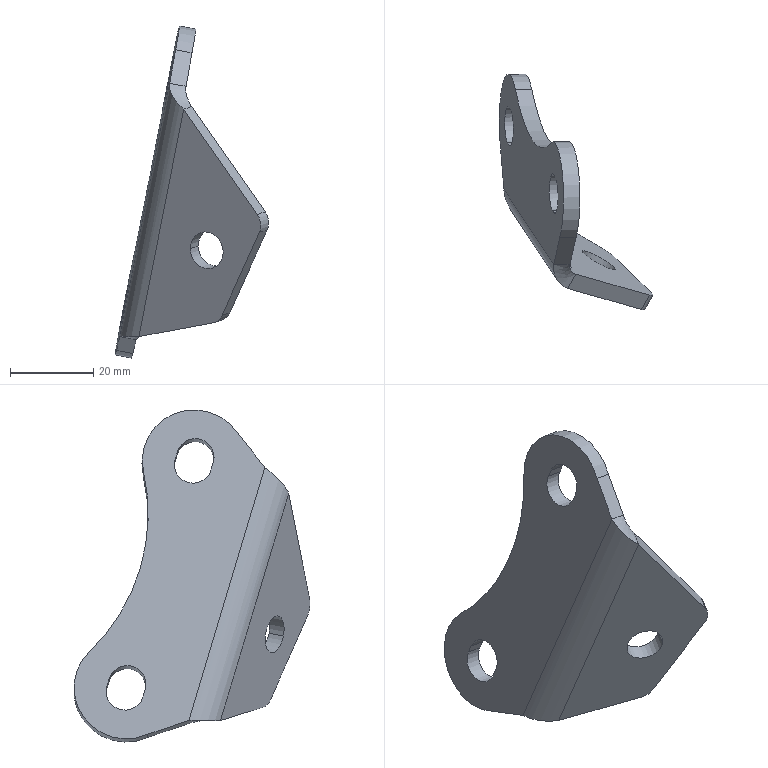Part | SolidWorks | features BaseBody 1 | 1 solid | 28 faces | box 36.914 x 56.808 x 79.896 mm | volume 12706 mm3 | plane 13 | cylinder 13 | spline 2 | commonest cylinder face diameters 9 x6 8 x3 25 x2 16 x1 94.633 x1
STEP:
#1=CARTESIAN_POINT('',(96.44,489.599,-664.758));
#2=VERTEX_POINT('',#1);
#3=CARTESIAN_POINT('',(96.779,498.232,-662.234));
#4=VERTEX_POINT('',#3);
#5=CARTESIAN_POINT('',(96.61,493.916,-663.496));
#6=DIRECTION('',(0.982,0.01648,-0.1883));
#7=DIRECTION('',(-0.03769,-0.9591,-0.2804));
#8=AXIS2_PLACEMENT_3D('',#5,#6,#7);
#9=CIRCLE('',#8,4.5);
#10=EDGE_CURVE('',#2,#4,#9,.T.);
#11=ORIENTED_EDGE('',*,*,#10,.F.);
#12=CARTESIAN_POINT('',(96.811,489.035,-662.876));
#13=VERTEX_POINT('',#12);
#14=CARTESIAN_POINT('',(96.811,489.035,-662.876));
#15=DIRECTION('',(-0.1852,0.2825,-0.9412));
#16=VECTOR('',#15,1000.);
#17=LINE('',#14,#16);
#18=EDGE_CURVE('',#13,#2,#17,.T.);
#19=ORIENTED_EDGE('',*,*,#18,.F.);
#20=CARTESIAN_POINT('',(97.15,497.667,-660.352));
#21=VERTEX_POINT('',#20);
#22=CARTESIAN_POINT('',(96.98,493.351,-661.614));
#23=DIRECTION('',(0.982,0.01648,-0.1883));
#24=DIRECTION('',(0.03769,0.9591,0.2804));
#25=AXIS2_PLACEMENT_3D('',#22,#23,#24);
#26=CIRCLE('',#25,4.5);
#27=EDGE_CURVE('',#21,#13,#26,.T.);
#28=ORIENTED_EDGE('',*,*,#27,.F.);
#29=CARTESIAN_POINT('',(96.779,498.232,-662.234));
#30=DIRECTION('',(0.1852,-0.2825,0.9412));
#31=VECTOR('',#30,1000.);
#32=LINE('',#29,#31);
#33=EDGE_CURVE('',#4,#21,#32,.T.);
#34=ORIENTED_EDGE('',*,*,#33,.F.);
#35=EDGE_LOOP('',(#11,#19,#28,#34));
#36=FACE_BOUND('',#35,.T.);
#37=CARTESIAN_POINT('',(85.696,505.984,-719.349));
#38=VERTEX_POINT('',#37);
#39=CARTESIAN_POINT('',(86.035,514.616,-716.825));
#40=VERTEX_POINT('',#39);
#41=CARTESIAN_POINT('',(85.866,510.3,-718.087));
#42=DIRECTION('',(0.982,0.01648,-0.1883));
#43=DIRECTION('',(-0.03769,-0.9591,-0.2804));
#44=AXIS2_PLACEMENT_3D('',#41,#42,#43);
#45=CIRCLE('',#44,4.5);
#46=EDGE_CURVE('',#38,#40,#45,.T.);
#47=ORIENTED_EDGE('',*,*,#46,.F.);
#48=CARTESIAN_POINT('',(86.067,505.419,-717.466));
#49=VERTEX_POINT('',#48);
#50=CARTESIAN_POINT('',(86.067,505.419,-717.466));
#51=DIRECTION('',(-0.1852,0.2825,-0.9412));
#52=VECTOR('',#51,1000.);
#53=LINE('',#50,#52);
#54=EDGE_CURVE('',#49,#38,#53,.T.);
#55=ORIENTED_EDGE('',*,*,#54,.F.);
#56=CARTESIAN_POINT('',(86.406,514.051,-714.942));
#57=VERTEX_POINT('',#56);
#58=CARTESIAN_POINT('',(86.236,509.735,-716.204));
#59=DIRECTION('',(0.982,0.01648,-0.1883));
#60=DIRECTION('',(0.03769,0.9591,0.2804));
#61=AXIS2_PLACEMENT_3D('',#58,#59,#60);
#62=CIRCLE('',#61,4.5);
#63=EDGE_CURVE('',#57,#49,#62,.T.);
#64=ORIENTED_EDGE('',*,*,#63,.F.);
#65=CARTESIAN_POINT('',(86.035,514.616,-716.825));
#66=DIRECTION('',(0.1852,-0.2825,0.9412));
#67=VECTOR('',#66,1000.);
#68=LINE('',#65,#67);
#69=EDGE_CURVE('',#40,#57,#68,.T.);
#70=ORIENTED_EDGE('',*,*,#69,.F.);
#71=EDGE_LOOP('',(#47,#55,#64,#70));
#72=FACE_BOUND('',#71,.T.);
#73=CARTESIAN_POINT('',(83.998,504.784,-728.31));
#74=VERTEX_POINT('',#73);
#75=CARTESIAN_POINT('',(84.798,494.924,-725.));
#76=VERTEX_POINT('',#75);
#77=CARTESIAN_POINT('',(83.998,504.784,-728.31));
#78=DIRECTION('',(0.0767,-0.9452,0.3173));
#79=VECTOR('',#78,1000.);
#80=LINE('',#77,#79);
#81=EDGE_CURVE('',#74,#76,#80,.T.);
#82=ORIENTED_EDGE('',*,*,#81,.F.);
#83=CARTESIAN_POINT('',(87.586,518.791,-708.376));
#84=VERTEX_POINT('',#83);
#85=CARTESIAN_POINT('',(86.051,510.017,-717.145));
#86=DIRECTION('',(-0.982,-0.01648,0.1883));
#87=DIRECTION('',(0.1228,0.7019,0.7016));
#88=AXIS2_PLACEMENT_3D('',#85,#86,#87);
#89=CIRCLE('',#88,12.5);
#90=EDGE_CURVE('',#84,#74,#89,.T.);
#91=ORIENTED_EDGE('',*,*,#90,.F.);
#92=CARTESIAN_POINT('',(96.084,505.831,-665.193));
#93=VERTEX_POINT('',#92);
#94=CARTESIAN_POINT('',(93.395,552.004,-675.178));
#95=DIRECTION('',(0.982,0.01648,-0.1883));
#96=DIRECTION('',(0.05684,-0.9758,0.211));
#97=AXIS2_PLACEMENT_3D('',#94,#95,#96);
#98=CIRCLE('',#97,47.317);
#99=EDGE_CURVE('',#93,#84,#98,.T.);
#100=ORIENTED_EDGE('',*,*,#99,.F.);
#101=CARTESIAN_POINT('',(98.228,483.083,-656.006));
#102=VERTEX_POINT('',#101);
#103=CARTESIAN_POINT('',(96.795,493.633,-662.555));
#104=DIRECTION('',(-0.982,-0.01648,0.1883));
#105=DIRECTION('',(0.1146,-0.844,0.5239));
#106=AXIS2_PLACEMENT_3D('',#103,#104,#105);
#107=CIRCLE('',#106,12.5);
#108=EDGE_CURVE('',#102,#93,#107,.T.);
#109=ORIENTED_EDGE('',*,*,#108,.F.);
#110=CARTESIAN_POINT('',(96.787,476.64,-664.082));
#111=VERTEX_POINT('',#110);
#112=CARTESIAN_POINT('',(96.787,476.64,-664.082));
#113=DIRECTION('',(0.1381,0.6176,0.7742));
#114=VECTOR('',#113,1000.);
#115=LINE('',#112,#114);
#116=EDGE_CURVE('',#111,#102,#115,.T.);
#117=ORIENTED_EDGE('',*,*,#116,.F.);
#118=CARTESIAN_POINT('',(96.787,476.64,-664.082));
#119=DIRECTION('',(-0.1852,0.2825,-0.9412));
#120=VECTOR('',#119,1000.);
#121=LINE('',#118,#120);
#122=EDGE_CURVE('',#111,#76,#121,.T.);
#123=ORIENTED_EDGE('',*,*,#122,.T.);
#124=EDGE_LOOP('',(#82,#91,#100,#109,#117,#123));
#125=FACE_OUTER_BOUND('',#124,.T.);
#126=CARTESIAN_POINT('',(80.679,518.209,-744.441));
#127=DIRECTION('',(0.982,0.01648,-0.1883));
#128=DIRECTION('',(0.,-0.9962,-0.08716));
#129=AXIS2_PLACEMENT_3D('',#126,#127,#128);
#130=PLANE('',#129);
#131=ADVANCED_FACE('',(#36,#72,#125),#130,.T.);
#132=CARTESIAN_POINT('',(98.124,474.285,-668.916));
#133=VERTEX_POINT('',#132);
#134=CARTESIAN_POINT('',(98.124,474.285,-668.916));
#135=CARTESIAN_POINT('',(97.917,474.34,-668.601));
#136=CARTESIAN_POINT('',(97.535,474.506,-667.961));
#137=CARTESIAN_POINT('',(97.089,474.899,-666.982));
#138=CARTESIAN_POINT('',(96.798,475.41,-665.999));
#139=CARTESIAN_POINT('',(96.683,476.003,-665.026));
#140=CARTESIAN_POINT('',(96.731,476.427,-664.393));
#141=CARTESIAN_POINT('',(96.787,476.64,-664.082));
#142=B_SPLINE_CURVE_WITH_KNOTS('',3,(#134,#135,#136,#137,#138,#139,#140,#141),.UNSPECIFIED.,.F.,.F.,(4,1,1,1,1,4),(0.,0.2,0.4,0.6,0.8,1.),.UNSPECIFIED.);
#143=EDGE_CURVE('',#133,#111,#142,.T.);
#144=ORIENTED_EDGE('',*,*,#143,.F.);
#145=CARTESIAN_POINT('',(87.359,490.701,-723.614));
#146=VERTEX_POINT('',#145);
#147=CARTESIAN_POINT('',(98.124,474.285,-668.916));
#148=DIRECTION('',(-0.1852,0.2825,-0.9412));
#149=VECTOR('',#148,1000.);
#150=LINE('',#147,#149);
#151=EDGE_CURVE('',#133,#146,#150,.T.);
#152=ORIENTED_EDGE('',*,*,#151,.T.);
#153=CARTESIAN_POINT('',(84.798,494.924,-725.));
#154=CARTESIAN_POINT('',(84.824,494.586,-724.896));
#155=CARTESIAN_POINT('',(84.938,493.913,-724.7));
#156=CARTESIAN_POINT('',(85.298,492.947,-724.429));
#157=CARTESIAN_POINT('',(85.834,492.063,-724.168));
#158=CARTESIAN_POINT('',(86.525,491.295,-723.903));
#159=CARTESIAN_POINT('',(87.071,490.881,-723.714));
#160=CARTESIAN_POINT('',(87.359,490.701,-723.614));
#161=B_SPLINE_CURVE_WITH_KNOTS('',3,(#153,#154,#155,#156,#157,#158,#159,#160),.UNSPECIFIED.,.F.,.F.,(4,1,1,1,1,4),(0.,0.2,0.4,0.6,0.8,1.),.UNSPECIFIED.);
#162=EDGE_CURVE('',#76,#146,#161,.T.);
#163=ORIENTED_EDGE('',*,*,#162,.F.);
#164=ORIENTED_EDGE('',*,*,#122,.F.);
#165=EDGE_LOOP('',(#144,#152,#163,#164));
#166=FACE_OUTER_BOUND('',#165,.T.);
#167=CARTESIAN_POINT('',(55.039,546.361,-896.917));
#168=DIRECTION('',(0.1852,-0.2825,0.9412));
#169=DIRECTION('',(-0.982,-0.01648,0.1883));
#170=AXIS2_PLACEMENT_3D('',#167,#168,#169);
#171=CYLINDRICAL_SURFACE('',#170,4.);
#172=ADVANCED_FACE('',(#166),#171,.F.);
#173=CARTESIAN_POINT('',(85.441,487.253,-724.271));
#174=VERTEX_POINT('',#173);
#175=CARTESIAN_POINT('',(85.441,487.253,-724.271));
#176=DIRECTION('',(0.4794,0.8621,0.1644));
#177=VECTOR('',#176,1000.);
#178=LINE('',#175,#177);
#179=EDGE_CURVE('',#174,#146,#178,.T.);
#180=ORIENTED_EDGE('',*,*,#179,.F.);
#181=CARTESIAN_POINT('',(80.87,494.858,-724.247));
#182=VERTEX_POINT('',#181);
#183=CARTESIAN_POINT('',(85.441,487.253,-724.271));
#184=CARTESIAN_POINT('',(84.901,487.556,-724.285));
#185=CARTESIAN_POINT('',(83.884,488.273,-724.29));
#186=CARTESIAN_POINT('',(82.612,489.64,-724.261));
#187=CARTESIAN_POINT('',(81.651,491.24,-724.223));
#188=CARTESIAN_POINT('',(81.041,493.004,-724.205));
#189=CARTESIAN_POINT('',(80.885,494.239,-724.225));
#190=CARTESIAN_POINT('',(80.87,494.858,-724.247));
#191=B_SPLINE_CURVE_WITH_KNOTS('',3,(#183,#184,#185,#186,#187,#188,#189,#190),.UNSPECIFIED.,.F.,.F.,(4,1,1,1,1,4),(0.,0.2,0.4,0.6,0.8,1.),.UNSPECIFIED.);
#192=EDGE_CURVE('',#174,#182,#191,.T.);
#193=ORIENTED_EDGE('',*,*,#192,.T.);
#194=CARTESIAN_POINT('',(84.798,494.924,-725.));
#195=DIRECTION('',(-0.982,-0.01648,0.1883));
#196=VECTOR('',#195,1000.);
#197=LINE('',#194,#196);
#198=EDGE_CURVE('',#76,#182,#197,.T.);
#199=ORIENTED_EDGE('',*,*,#198,.F.);
#200=ORIENTED_EDGE('',*,*,#162,.T.);
#201=EDGE_LOOP('',(#180,#193,#199,#200));
#202=FACE_OUTER_BOUND('',#201,.T.);
#203=CARTESIAN_POINT('',(84.908,495.037,-725.059));
#204=CARTESIAN_POINT('',(83.522,495.047,-724.784));
#205=CARTESIAN_POINT('',(82.136,495.058,-724.508));
#206=CARTESIAN_POINT('',(80.75,495.068,-724.232));
#207=CARTESIAN_POINT('',(84.91,495.,-725.047));
#208=CARTESIAN_POINT('',(83.523,494.999,-724.775));
#209=CARTESIAN_POINT('',(82.137,494.998,-724.502));
#210=CARTESIAN_POINT('',(80.75,494.997,-724.229));
#211=CARTESIAN_POINT('',(84.935,494.634,-724.928));
#212=CARTESIAN_POINT('',(83.543,494.522,-724.687));
#213=CARTESIAN_POINT('',(82.15,494.411,-724.446));
#214=CARTESIAN_POINT('',(80.758,494.3,-724.206));
#215=CARTESIAN_POINT('',(85.055,493.94,-724.715));
#216=CARTESIAN_POINT('',(83.678,493.619,-724.54));
#217=CARTESIAN_POINT('',(82.301,493.298,-724.365));
#218=CARTESIAN_POINT('',(80.924,492.977,-724.191));
#219=CARTESIAN_POINT('',(85.408,492.998,-724.435));
#220=CARTESIAN_POINT('',(84.119,492.395,-724.363));
#221=CARTESIAN_POINT('',(82.83,491.792,-724.29));
#222=CARTESIAN_POINT('',(81.542,491.189,-724.217));
#223=CARTESIAN_POINT('',(85.931,492.135,-724.165));
#224=CARTESIAN_POINT('',(84.792,491.279,-724.198));
#225=CARTESIAN_POINT('',(83.654,490.423,-724.231));
#226=CARTESIAN_POINT('',(82.516,489.567,-724.264));
#227=CARTESIAN_POINT('',(86.604,491.386,-723.891));
#228=CARTESIAN_POINT('',(85.671,490.318,-724.028));
#229=CARTESIAN_POINT('',(84.738,489.25,-724.165));
#230=CARTESIAN_POINT('',(83.805,488.182,-724.302));
#231=CARTESIAN_POINT('',(87.166,490.958,-723.685));
#232=CARTESIAN_POINT('',(86.409,489.777,-723.891));
#233=CARTESIAN_POINT('',(85.652,488.596,-724.096));
#234=CARTESIAN_POINT('',(84.895,487.415,-724.302));
#235=CARTESIAN_POINT('',(87.48,490.766,-723.571));
#236=CARTESIAN_POINT('',(86.823,489.537,-723.81));
#237=CARTESIAN_POINT('',(86.165,488.309,-724.049));
#238=CARTESIAN_POINT('',(85.508,487.081,-724.288));
#239=CARTESIAN_POINT('',(87.512,490.746,-723.559));
#240=CARTESIAN_POINT('',(86.865,489.514,-723.802));
#241=CARTESIAN_POINT('',(86.218,488.281,-724.044));
#242=CARTESIAN_POINT('',(85.571,487.048,-724.287));
#243=B_SPLINE_SURFACE_WITH_KNOTS('',3,3,((#203,#204,#205,#206),(#207,#208,#209,#210),(#211,#212,#213,#214),(#215,#216,#217,#218),(#219,#220,#221,#222),(#223,#224,#225,#226),(#227,#228,#229,#230),(#231,#232,#233,#234),(#235,#236,#237,#238),(#239,#240,#241,#242)),.UNSPECIFIED.,.F.,.F.,.F.,(4,1,1,1,1,1,1,4),(4,4),(-0.02261,0.,0.2,0.4,0.6,0.8,1.,1.023),(-0.03,1.03),.UNSPECIFIED.);
#244=ADVANCED_FACE('',(#202),#243,.T.);
#245=ORIENTED_EDGE('',*,*,#198,.T.);
#246=CARTESIAN_POINT('',(80.07,504.718,-727.557));
#247=VERTEX_POINT('',#246);
#248=CARTESIAN_POINT('',(80.87,494.858,-724.247));
#249=DIRECTION('',(-0.0767,0.9452,-0.3173));
#250=VECTOR('',#249,1000.);
#251=LINE('',#248,#250);
#252=EDGE_CURVE('',#182,#247,#251,.T.);
#253=ORIENTED_EDGE('',*,*,#252,.T.);
#254=CARTESIAN_POINT('',(80.07,504.718,-727.557));
#255=DIRECTION('',(0.982,0.01648,-0.1883));
#256=VECTOR('',#255,1000.);
#257=LINE('',#254,#256);
#258=EDGE_CURVE('',#247,#74,#257,.T.);
#259=ORIENTED_EDGE('',*,*,#258,.T.);
#260=ORIENTED_EDGE('',*,*,#81,.T.);
#261=EDGE_LOOP('',(#245,#253,#259,#260));
#262=FACE_OUTER_BOUND('',#261,.T.);
#263=CARTESIAN_POINT('',(82.434,499.821,-726.279));
#264=DIRECTION('',(-0.1728,-0.326,-0.9295));
#265=DIRECTION('',(0.,-0.9436,0.331));
#266=AXIS2_PLACEMENT_3D('',#263,#264,#265);
#267=PLANE('',#266);
#268=ADVANCED_FACE('',(#262),#267,.T.);
#269=ORIENTED_EDGE('',*,*,#258,.F.);
#270=CARTESIAN_POINT('',(83.658,518.725,-707.622));
#271=VERTEX_POINT('',#270);
#272=CARTESIAN_POINT('',(82.123,509.951,-716.392));
#273=DIRECTION('',(0.982,0.01648,-0.1883));
#274=DIRECTION('',(-0.1643,-0.4187,-0.8931));
#275=AXIS2_PLACEMENT_3D('',#272,#273,#274);
#276=CIRCLE('',#275,12.5);
#277=EDGE_CURVE('',#247,#271,#276,.T.);
#278=ORIENTED_EDGE('',*,*,#277,.T.);
#279=CARTESIAN_POINT('',(83.658,518.725,-707.622));
#280=DIRECTION('',(0.982,0.01648,-0.1883));
#281=VECTOR('',#280,1000.);
#282=LINE('',#279,#281);
#283=EDGE_CURVE('',#271,#84,#282,.T.);
#284=ORIENTED_EDGE('',*,*,#283,.T.);
#285=ORIENTED_EDGE('',*,*,#90,.T.);
#286=EDGE_LOOP('',(#269,#278,#284,#285));
#287=FACE_OUTER_BOUND('',#286,.T.);
#288=CARTESIAN_POINT('',(84.087,509.984,-716.769));
#289=DIRECTION('',(0.982,0.01648,-0.1883));
#290=DIRECTION('',(-0.1643,-0.4187,-0.8931));
#291=AXIS2_PLACEMENT_3D('',#288,#289,#290);
#292=CYLINDRICAL_SURFACE('',#291,12.5);
#293=ADVANCED_FACE('',(#287),#292,.T.);
#294=ORIENTED_EDGE('',*,*,#283,.F.);
#295=CARTESIAN_POINT('',(92.157,505.765,-664.44));
#296=VERTEX_POINT('',#295);
#297=CARTESIAN_POINT('',(89.467,551.938,-674.425));
#298=DIRECTION('',(-0.982,-0.01648,0.1883));
#299=DIRECTION('',(-0.1228,-0.7019,-0.7016));
#300=AXIS2_PLACEMENT_3D('',#297,#298,#299);
#301=CIRCLE('',#300,47.317);
#302=EDGE_CURVE('',#271,#296,#301,.T.);
#303=ORIENTED_EDGE('',*,*,#302,.T.);
#304=CARTESIAN_POINT('',(92.157,505.765,-664.44));
#305=DIRECTION('',(0.982,0.01648,-0.1883));
#306=VECTOR('',#305,1000.);
#307=LINE('',#304,#306);
#308=EDGE_CURVE('',#296,#93,#307,.T.);
#309=ORIENTED_EDGE('',*,*,#308,.T.);
#310=ORIENTED_EDGE('',*,*,#99,.T.);
#311=EDGE_LOOP('',(#294,#303,#309,#310));
#312=FACE_OUTER_BOUND('',#311,.T.);
#313=CARTESIAN_POINT('',(91.431,551.971,-674.802));
#314=DIRECTION('',(-0.982,-0.01648,0.1883));
#315=DIRECTION('',(-0.1228,-0.7019,-0.7016));
#316=AXIS2_PLACEMENT_3D('',#313,#314,#315);
#317=CYLINDRICAL_SURFACE('',#316,47.317);
#318=ADVANCED_FACE('',(#312),#317,.F.);
#319=ORIENTED_EDGE('',*,*,#308,.F.);
#320=CARTESIAN_POINT('',(94.3,483.017,-655.253));
#321=VERTEX_POINT('',#320);
#322=CARTESIAN_POINT('',(92.867,493.567,-661.802));
#323=DIRECTION('',(0.982,0.01648,-0.1883));
#324=DIRECTION('',(-0.05684,0.9758,-0.211));
#325=AXIS2_PLACEMENT_3D('',#322,#323,#324);
#326=CIRCLE('',#325,12.5);
#327=EDGE_CURVE('',#296,#321,#326,.T.);
#328=ORIENTED_EDGE('',*,*,#327,.T.);
#329=CARTESIAN_POINT('',(98.228,483.083,-656.006));
#330=DIRECTION('',(-0.982,-0.01648,0.1883));
#331=VECTOR('',#330,1000.);
#332=LINE('',#329,#331);
#333=EDGE_CURVE('',#102,#321,#332,.T.);
#334=ORIENTED_EDGE('',*,*,#333,.F.);
#335=ORIENTED_EDGE('',*,*,#108,.T.);
#336=EDGE_LOOP('',(#319,#328,#334,#335));
#337=FACE_OUTER_BOUND('',#336,.T.);
#338=CARTESIAN_POINT('',(94.831,493.6,-662.178));
#339=DIRECTION('',(0.982,0.01648,-0.1883));
#340=DIRECTION('',(-0.05684,0.9758,-0.211));
#341=AXIS2_PLACEMENT_3D('',#338,#339,#340);
#342=CYLINDRICAL_SURFACE('',#341,12.5);
#343=ADVANCED_FACE('',(#337),#342,.T.);
#344=ORIENTED_EDGE('',*,*,#333,.T.);
#345=CARTESIAN_POINT('',(92.859,476.574,-663.329));
#346=VERTEX_POINT('',#345);
#347=CARTESIAN_POINT('',(94.3,483.017,-655.253));
#348=DIRECTION('',(-0.1381,-0.6176,-0.7742));
#349=VECTOR('',#348,1000.);
#350=LINE('',#347,#349);
#351=EDGE_CURVE('',#321,#346,#350,.T.);
#352=ORIENTED_EDGE('',*,*,#351,.T.);
#353=CARTESIAN_POINT('',(92.859,476.574,-663.329));
#354=DIRECTION('',(0.982,0.01648,-0.1883));
#355=VECTOR('',#354,1000.);
#356=LINE('',#353,#355);
#357=EDGE_CURVE('',#346,#111,#356,.T.);
#358=ORIENTED_EDGE('',*,*,#357,.T.);
#359=ORIENTED_EDGE('',*,*,#116,.T.);
#360=EDGE_LOOP('',(#344,#352,#358,#359));
#361=FACE_OUTER_BOUND('',#360,.T.);
#362=CARTESIAN_POINT('',(95.544,479.829,-659.667));
#363=DIRECTION('',(0.1291,-0.7863,0.6042));
#364=DIRECTION('',(-0.9868,-0.162,0.));
#365=AXIS2_PLACEMENT_3D('',#362,#363,#364);
#366=PLANE('',#365);
#367=ADVANCED_FACE('',(#361),#366,.T.);
#368=ORIENTED_EDGE('',*,*,#357,.F.);
#369=CARTESIAN_POINT('',(96.206,470.837,-669.574));
#370=VERTEX_POINT('',#369);
#371=CARTESIAN_POINT('',(92.859,476.574,-663.329));
#372=CARTESIAN_POINT('',(92.792,476.08,-663.722));
#373=CARTESIAN_POINT('',(92.786,475.094,-664.531));
#374=CARTESIAN_POINT('',(93.151,473.703,-665.793));
#375=CARTESIAN_POINT('',(93.867,472.477,-667.076));
#376=CARTESIAN_POINT('',(94.894,471.483,-668.349));
#377=CARTESIAN_POINT('',(95.748,471.015,-669.172));
#378=CARTESIAN_POINT('',(96.206,470.837,-669.574));
#379=B_SPLINE_CURVE_WITH_KNOTS('',3,(#371,#372,#373,#374,#375,#376,#377,#378),.UNSPECIFIED.,.F.,.F.,(4,1,1,1,1,4),(0.,0.2,0.4,0.6,0.8,1.),.UNSPECIFIED.);
#380=EDGE_CURVE('',#346,#370,#379,.T.);
#381=ORIENTED_EDGE('',*,*,#380,.T.);
#382=CARTESIAN_POINT('',(98.124,474.285,-668.916));
#383=DIRECTION('',(-0.4794,-0.8621,-0.1644));
#384=VECTOR('',#383,1000.);
#385=LINE('',#382,#384);
#386=EDGE_CURVE('',#133,#370,#385,.T.);
#387=ORIENTED_EDGE('',*,*,#386,.F.);
#388=ORIENTED_EDGE('',*,*,#143,.T.);
#389=EDGE_LOOP('',(#368,#381,#387,#388));
#390=FACE_OUTER_BOUND('',#389,.T.);
#391=CARTESIAN_POINT('',(98.245,474.373,-668.995));
#392=CARTESIAN_POINT('',(97.595,473.142,-669.237));
#393=CARTESIAN_POINT('',(96.946,471.91,-669.479));
#394=CARTESIAN_POINT('',(96.297,470.678,-669.72));
#395=CARTESIAN_POINT('',(98.223,474.378,-668.962));
#396=CARTESIAN_POINT('',(97.565,473.151,-669.201));
#397=CARTESIAN_POINT('',(96.906,471.923,-669.439));
#398=CARTESIAN_POINT('',(96.247,470.696,-669.678));
#399=CARTESIAN_POINT('',(98.002,474.432,-668.618));
#400=CARTESIAN_POINT('',(97.244,473.251,-668.823));
#401=CARTESIAN_POINT('',(96.486,472.071,-669.028));
#402=CARTESIAN_POINT('',(95.729,470.89,-669.233));
#403=CARTESIAN_POINT('',(97.614,474.596,-667.95));
#404=CARTESIAN_POINT('',(96.681,473.528,-668.086));
#405=CARTESIAN_POINT('',(95.748,472.46,-668.223));
#406=CARTESIAN_POINT('',(94.815,471.393,-668.36));
#407=CARTESIAN_POINT('',(97.186,474.972,-666.98));
#408=CARTESIAN_POINT('',(96.047,474.116,-667.013));
#409=CARTESIAN_POINT('',(94.909,473.26,-667.045));
#410=CARTESIAN_POINT('',(93.77,472.404,-667.078));
#411=CARTESIAN_POINT('',(96.908,475.461,-666.005));
#412=CARTESIAN_POINT('',(95.619,474.858,-665.933));
#413=CARTESIAN_POINT('',(94.33,474.255,-665.86));
#414=CARTESIAN_POINT('',(93.041,473.652,-665.787));
#415=CARTESIAN_POINT('',(96.8,476.03,-665.04));
#416=CARTESIAN_POINT('',(95.423,475.709,-664.866));
#417=CARTESIAN_POINT('',(94.046,475.388,-664.691));
#418=CARTESIAN_POINT('',(92.669,475.067,-664.516));
#419=CARTESIAN_POINT('',(96.852,476.459,-664.38));
#420=CARTESIAN_POINT('',(95.46,476.347,-664.139));
#421=CARTESIAN_POINT('',(94.067,476.235,-663.899));
#422=CARTESIAN_POINT('',(92.675,476.123,-663.659));
#423=CARTESIAN_POINT('',(96.917,476.685,-664.04));
#424=CARTESIAN_POINT('',(95.53,476.683,-663.768));
#425=CARTESIAN_POINT('',(94.143,476.68,-663.496));
#426=CARTESIAN_POINT('',(92.756,476.678,-663.223));
#427=CARTESIAN_POINT('',(96.924,476.707,-664.008));
#428=CARTESIAN_POINT('',(95.537,476.715,-663.733));
#429=CARTESIAN_POINT('',(94.151,476.723,-663.457));
#430=CARTESIAN_POINT('',(92.765,476.731,-663.182));
#431=B_SPLINE_SURFACE_WITH_KNOTS('',3,3,((#391,#392,#393,#394),(#395,#396,#397,#398),(#399,#400,#401,#402),(#403,#404,#405,#406),(#407,#408,#409,#410),(#411,#412,#413,#414),(#415,#416,#417,#418),(#419,#420,#421,#422),(#423,#424,#425,#426),(#427,#428,#429,#430)),.UNSPECIFIED.,.F.,.F.,.F.,(4,1,1,1,1,1,1,4),(4,4),(-0.02103,0.,0.2,0.4,0.6,0.8,1.,1.021),(-0.03,1.03),.UNSPECIFIED.);
#432=ADVANCED_FACE('',(#390),#431,.T.);
#433=CARTESIAN_POINT('',(115.847,469.261,-694.252));
#434=VERTEX_POINT('',#433);
#435=CARTESIAN_POINT('',(115.847,469.261,-694.252));
#436=DIRECTION('',(-0.5658,0.1604,0.8088));
#437=VECTOR('',#436,1000.);
#438=LINE('',#435,#437);
#439=EDGE_CURVE('',#434,#133,#438,.T.);
#440=ORIENTED_EDGE('',*,*,#439,.T.);
#441=ORIENTED_EDGE('',*,*,#386,.T.);
#442=CARTESIAN_POINT('',(113.93,465.812,-694.91));
#443=VERTEX_POINT('',#442);
#444=CARTESIAN_POINT('',(96.206,470.837,-669.574));
#445=DIRECTION('',(0.5658,-0.1604,-0.8088));
#446=VECTOR('',#445,1000.);
#447=LINE('',#444,#446);
#448=EDGE_CURVE('',#370,#443,#447,.T.);
#449=ORIENTED_EDGE('',*,*,#448,.T.);
#450=CARTESIAN_POINT('',(113.93,465.812,-694.91));
#451=DIRECTION('',(0.4794,0.8621,0.1644));
#452=VECTOR('',#451,1000.);
#453=LINE('',#450,#452);
#454=EDGE_CURVE('',#443,#434,#453,.T.);
#455=ORIENTED_EDGE('',*,*,#454,.T.);
#456=EDGE_LOOP('',(#440,#441,#449,#455));
#457=FACE_OUTER_BOUND('',#456,.T.);
#458=CARTESIAN_POINT('',(106.76,469.841,-682.961));
#459=DIRECTION('',(0.6709,-0.4807,0.5646));
#460=DIRECTION('',(0.,-0.7614,-0.6483));
#461=AXIS2_PLACEMENT_3D('',#458,#459,#460);
#462=PLANE('',#461);
#463=ADVANCED_FACE('',(#457),#462,.T.);
#464=ORIENTED_EDGE('',*,*,#454,.F.);
#465=CARTESIAN_POINT('',(114.409,466.364,-699.198));
#466=VERTEX_POINT('',#465);
#467=CARTESIAN_POINT('',(111.246,467.735,-697.168));
#468=DIRECTION('',(0.4794,0.8621,0.1644));
#469=DIRECTION('',(0.6709,-0.4807,0.5646));
#470=AXIS2_PLACEMENT_3D('',#467,#468,#469);
#471=CIRCLE('',#470,4.);
#472=EDGE_CURVE('',#443,#466,#471,.T.);
#473=ORIENTED_EDGE('',*,*,#472,.T.);
#474=CARTESIAN_POINT('',(116.326,469.812,-698.54));
#475=VERTEX_POINT('',#474);
#476=CARTESIAN_POINT('',(116.326,469.812,-698.54));
#477=DIRECTION('',(-0.4794,-0.8621,-0.1644));
#478=VECTOR('',#477,1000.);
#479=LINE('',#476,#478);
#480=EDGE_CURVE('',#475,#466,#479,.T.);
#481=ORIENTED_EDGE('',*,*,#480,.F.);
#482=CARTESIAN_POINT('',(113.164,471.183,-696.511));
#483=DIRECTION('',(-0.4794,-0.8621,-0.1644));
#484=DIRECTION('',(0.7906,-0.3429,-0.5073));
#485=AXIS2_PLACEMENT_3D('',#482,#483,#484);
#486=CIRCLE('',#485,4.);
#487=EDGE_CURVE('',#475,#434,#486,.T.);
#488=ORIENTED_EDGE('',*,*,#487,.T.);
#489=EDGE_LOOP('',(#464,#473,#481,#488));
#490=FACE_OUTER_BOUND('',#489,.T.);
#491=CARTESIAN_POINT('',(59.432,374.559,-714.936));
#492=DIRECTION('',(0.4794,0.8621,0.1644));
#493=DIRECTION('',(0.6709,-0.4807,0.5646));
#494=AXIS2_PLACEMENT_3D('',#491,#492,#493);
#495=CYLINDRICAL_SURFACE('',#494,4.);
#496=ADVANCED_FACE('',(#490),#495,.T.);
#497=CARTESIAN_POINT('',(107.628,475.551,-703.269));
#498=VERTEX_POINT('',#497);
#499=CARTESIAN_POINT('',(99.729,479.789,-702.46));
#500=VERTEX_POINT('',#499);
#501=CARTESIAN_POINT('',(103.679,477.67,-702.865));
#502=DIRECTION('',(0.4794,0.8621,0.1644));
#503=DIRECTION('',(0.8776,-0.4709,-0.08979));
#504=AXIS2_PLACEMENT_3D('',#501,#502,#503);
#505=CIRCLE('',#504,4.5);
#506=EDGE_CURVE('',#498,#500,#505,.T.);
#507=ORIENTED_EDGE('',*,*,#506,.F.);
#508=CARTESIAN_POINT('',(103.679,477.67,-702.865));
#509=DIRECTION('',(0.4794,0.8621,0.1644));
#510=DIRECTION('',(-0.8776,0.4709,0.08979));
#511=AXIS2_PLACEMENT_3D('',#508,#509,#510);
#512=CIRCLE('',#511,4.5);
#513=EDGE_CURVE('',#500,#498,#512,.T.);
#514=ORIENTED_EDGE('',*,*,#513,.F.);
#515=EDGE_LOOP('',(#507,#514));
#516=FACE_BOUND('',#515,.T.);
#517=CARTESIAN_POINT('',(107.354,478.6,-718.462));
#518=VERTEX_POINT('',#517);
#519=CARTESIAN_POINT('',(107.354,478.6,-718.462));
#520=DIRECTION('',(0.381,-0.3732,0.8459));
#521=VECTOR('',#520,1000.);
#522=LINE('',#519,#521);
#523=EDGE_CURVE('',#518,#475,#522,.T.);
#524=ORIENTED_EDGE('',*,*,#523,.F.);
#525=CARTESIAN_POINT('',(105.066,480.228,-720.328));
#526=VERTEX_POINT('',#525);
#527=CARTESIAN_POINT('',(104.192,479.971,-716.433));
#528=DIRECTION('',(-0.4794,-0.8621,-0.1644));
#529=DIRECTION('',(0.2186,0.06411,-0.9737));
#530=AXIS2_PLACEMENT_3D('',#527,#528,#529);
#531=CIRCLE('',#530,4.);
#532=EDGE_CURVE('',#526,#518,#531,.T.);
#533=ORIENTED_EDGE('',*,*,#532,.F.);
#534=CARTESIAN_POINT('',(87.359,490.701,-723.614));
#535=DIRECTION('',(0.8499,-0.5027,0.1577));
#536=VECTOR('',#535,1000.);
#537=LINE('',#534,#536);
#538=EDGE_CURVE('',#146,#526,#537,.T.);
#539=ORIENTED_EDGE('',*,*,#538,.F.);
#540=ORIENTED_EDGE('',*,*,#151,.F.);
#541=ORIENTED_EDGE('',*,*,#439,.F.);
#542=ORIENTED_EDGE('',*,*,#487,.F.);
#543=EDGE_LOOP('',(#524,#533,#539,#540,#541,#542));
#544=FACE_OUTER_BOUND('',#543,.T.);
#545=CARTESIAN_POINT('',(165.843,298.231,56.868));
#546=DIRECTION('',(0.4794,0.8621,0.1644));
#547=DIRECTION('',(0.3244,0.,-0.9459));
#548=AXIS2_PLACEMENT_3D('',#545,#546,#547);
#549=PLANE('',#548);
#550=ADVANCED_FACE('',(#516,#544),#549,.T.);
#551=CARTESIAN_POINT('',(103.149,476.78,-720.985));
#552=VERTEX_POINT('',#551);
#553=CARTESIAN_POINT('',(103.149,476.78,-720.985));
#554=DIRECTION('',(-0.8499,0.5027,-0.1577));
#555=VECTOR('',#554,1000.);
#556=LINE('',#553,#555);
#557=EDGE_CURVE('',#552,#174,#556,.T.);
#558=ORIENTED_EDGE('',*,*,#557,.T.);
#559=ORIENTED_EDGE('',*,*,#179,.T.);
#560=ORIENTED_EDGE('',*,*,#538,.T.);
#561=CARTESIAN_POINT('',(105.066,480.228,-720.328));
#562=DIRECTION('',(-0.4794,-0.8621,-0.1644));
#563=VECTOR('',#562,1000.);
#564=LINE('',#561,#563);
#565=EDGE_CURVE('',#526,#552,#564,.T.);
#566=ORIENTED_EDGE('',*,*,#565,.T.);
#567=EDGE_LOOP('',(#558,#559,#560,#566));
#568=FACE_OUTER_BOUND('',#567,.T.);
#569=CARTESIAN_POINT('',(96.044,483.273,-722.153));
#570=DIRECTION('',(0.2186,0.06411,-0.9737));
#571=DIRECTION('',(0.,-0.9978,-0.0657));
#572=AXIS2_PLACEMENT_3D('',#569,#570,#571);
#573=PLANE('',#572);
#574=ADVANCED_FACE('',(#568),#573,.T.);
#575=CARTESIAN_POINT('',(105.437,475.152,-719.12));
#576=VERTEX_POINT('',#575);
#577=CARTESIAN_POINT('',(105.437,475.152,-719.12));
#578=DIRECTION('',(0.4794,0.8621,0.1644));
#579=VECTOR('',#578,1000.);
#580=LINE('',#577,#579);
#581=EDGE_CURVE('',#576,#518,#580,.T.);
#582=ORIENTED_EDGE('',*,*,#581,.F.);
#583=CARTESIAN_POINT('',(102.274,476.523,-717.09));
#584=DIRECTION('',(0.4794,0.8621,0.1644));
#585=DIRECTION('',(0.7906,-0.3429,-0.5073));
#586=AXIS2_PLACEMENT_3D('',#583,#584,#585);
#587=CIRCLE('',#586,4.);
#588=EDGE_CURVE('',#576,#552,#587,.T.);
#589=ORIENTED_EDGE('',*,*,#588,.T.);
#590=ORIENTED_EDGE('',*,*,#565,.F.);
#591=ORIENTED_EDGE('',*,*,#532,.T.);
#592=EDGE_LOOP('',(#582,#589,#590,#591));
#593=FACE_OUTER_BOUND('',#592,.T.);
#594=CARTESIAN_POINT('',(45.573,374.559,-736.533));
#595=DIRECTION('',(0.4794,0.8621,0.1644));
#596=DIRECTION('',(0.7906,-0.3429,-0.5073));
#597=AXIS2_PLACEMENT_3D('',#594,#595,#596);
#598=CYLINDRICAL_SURFACE('',#597,4.);
#599=ADVANCED_FACE('',(#593),#598,.T.);
#600=CARTESIAN_POINT('',(97.812,476.34,-703.118));
#601=VERTEX_POINT('',#600);
#602=CARTESIAN_POINT('',(105.71,472.102,-703.926));
#603=VERTEX_POINT('',#602);
#604=CARTESIAN_POINT('',(101.761,474.221,-703.522));
#605=DIRECTION('',(-0.4794,-0.8621,-0.1644));
#606=DIRECTION('',(-0.8776,0.4709,0.08979));
#607=AXIS2_PLACEMENT_3D('',#604,#605,#606);
#608=CIRCLE('',#607,4.5);
#609=EDGE_CURVE('',#601,#603,#608,.T.);
#610=ORIENTED_EDGE('',*,*,#609,.F.);
#611=CARTESIAN_POINT('',(101.761,474.221,-703.522));
#612=DIRECTION('',(-0.4794,-0.8621,-0.1644));
#613=DIRECTION('',(0.8776,-0.4709,-0.08979));
#614=AXIS2_PLACEMENT_3D('',#611,#612,#613);
#615=CIRCLE('',#614,4.5);
#616=EDGE_CURVE('',#603,#601,#615,.T.);
#617=ORIENTED_EDGE('',*,*,#616,.F.);
#618=EDGE_LOOP('',(#610,#617));
#619=FACE_BOUND('',#618,.T.);
#620=ORIENTED_EDGE('',*,*,#448,.F.);
#621=CARTESIAN_POINT('',(85.441,487.253,-724.271));
#622=DIRECTION('',(0.1852,-0.2825,0.9412));
#623=VECTOR('',#622,1000.);
#624=LINE('',#621,#623);
#625=EDGE_CURVE('',#174,#370,#624,.T.);
#626=ORIENTED_EDGE('',*,*,#625,.F.);
#627=ORIENTED_EDGE('',*,*,#557,.F.);
#628=ORIENTED_EDGE('',*,*,#588,.F.);
#629=CARTESIAN_POINT('',(114.409,466.364,-699.198));
#630=DIRECTION('',(-0.381,0.3732,-0.8459));
#631=VECTOR('',#630,1000.);
#632=LINE('',#629,#631);
#633=EDGE_CURVE('',#466,#576,#632,.T.);
#634=ORIENTED_EDGE('',*,*,#633,.F.);
#635=ORIENTED_EDGE('',*,*,#472,.F.);
#636=EDGE_LOOP('',(#620,#626,#627,#628,#634,#635));
#637=FACE_OUTER_BOUND('',#636,.T.);
#638=CARTESIAN_POINT('',(163.925,294.782,56.211));
#639=DIRECTION('',(0.4794,0.8621,0.1644));
#640=DIRECTION('',(0.3244,0.,-0.9459));
#641=AXIS2_PLACEMENT_3D('',#638,#639,#640);
#642=PLANE('',#641);
#643=ADVANCED_FACE('',(#619,#637),#642,.F.);
#644=ORIENTED_EDGE('',*,*,#633,.T.);
#645=ORIENTED_EDGE('',*,*,#581,.T.);
#646=ORIENTED_EDGE('',*,*,#523,.T.);
#647=ORIENTED_EDGE('',*,*,#480,.T.);
#648=EDGE_LOOP('',(#644,#645,#646,#647));
#649=FACE_OUTER_BOUND('',#648,.T.);
#650=CARTESIAN_POINT('',(111.021,472.345,-708.52));
#651=DIRECTION('',(0.7906,-0.3429,-0.5073));
#652=DIRECTION('',(0.,-0.8285,0.56));
#653=AXIS2_PLACEMENT_3D('',#650,#651,#652);
#654=PLANE('',#653);
#655=ADVANCED_FACE('',(#649),#654,.T.);
#656=ORIENTED_EDGE('',*,*,#192,.F.);
#657=ORIENTED_EDGE('',*,*,#625,.T.);
#658=ORIENTED_EDGE('',*,*,#380,.F.);
#659=CARTESIAN_POINT('',(80.87,494.858,-724.247));
#660=DIRECTION('',(0.1852,-0.2825,0.9412));
#661=VECTOR('',#660,1000.);
#662=LINE('',#659,#661);
#663=EDGE_CURVE('',#182,#346,#662,.T.);
#664=ORIENTED_EDGE('',*,*,#663,.F.);
#665=EDGE_LOOP('',(#656,#657,#658,#664));
#666=FACE_OUTER_BOUND('',#665,.T.);
#667=CARTESIAN_POINT('',(55.039,546.361,-896.917));
#668=DIRECTION('',(0.1852,-0.2825,0.9412));
#669=DIRECTION('',(-0.982,-0.01648,0.1883));
#670=AXIS2_PLACEMENT_3D('',#667,#668,#669);
#671=CYLINDRICAL_SURFACE('',#670,8.);
#672=ADVANCED_FACE('',(#666),#671,.T.);
#673=CARTESIAN_POINT('',(92.883,488.969,-662.123));
#674=VERTEX_POINT('',#673);
#675=CARTESIAN_POINT('',(93.222,497.601,-659.599));
#676=VERTEX_POINT('',#675);
#677=CARTESIAN_POINT('',(93.052,493.285,-660.861));
#678=DIRECTION('',(-0.982,-0.01648,0.1883));
#679=DIRECTION('',(-0.03769,-0.9591,-0.2804));
#680=AXIS2_PLACEMENT_3D('',#677,#678,#679);
#681=CIRCLE('',#680,4.5);
#682=EDGE_CURVE('',#674,#676,#681,.T.);
#683=ORIENTED_EDGE('',*,*,#682,.F.);
#684=CARTESIAN_POINT('',(92.512,489.534,-664.005));
#685=VERTEX_POINT('',#684);
#686=CARTESIAN_POINT('',(92.883,488.969,-662.123));
#687=DIRECTION('',(-0.1852,0.2825,-0.9412));
#688=VECTOR('',#687,1000.);
#689=LINE('',#686,#688);
#690=EDGE_CURVE('',#674,#685,#689,.T.);
#691=ORIENTED_EDGE('',*,*,#690,.T.);
#692=CARTESIAN_POINT('',(92.852,498.166,-661.481));
#693=VERTEX_POINT('',#692);
#694=CARTESIAN_POINT('',(92.682,493.85,-662.743));
#695=DIRECTION('',(-0.982,-0.01648,0.1883));
#696=DIRECTION('',(0.03769,0.9591,0.2804));
#697=AXIS2_PLACEMENT_3D('',#694,#695,#696);
#698=CIRCLE('',#697,4.5);
#699=EDGE_CURVE('',#693,#685,#698,.T.);
#700=ORIENTED_EDGE('',*,*,#699,.F.);
#701=CARTESIAN_POINT('',(92.852,498.166,-661.481));
#702=DIRECTION('',(0.1852,-0.2825,0.9412));
#703=VECTOR('',#702,1000.);
#704=LINE('',#701,#703);
#705=EDGE_CURVE('',#693,#676,#704,.T.);
#706=ORIENTED_EDGE('',*,*,#705,.T.);
#707=EDGE_LOOP('',(#683,#691,#700,#706));
#708=FACE_BOUND('',#707,.T.);
#709=CARTESIAN_POINT('',(82.139,505.353,-716.713));
#710=VERTEX_POINT('',#709);
#711=CARTESIAN_POINT('',(82.478,513.985,-714.189));
#712=VERTEX_POINT('',#711);
#713=CARTESIAN_POINT('',(82.308,509.669,-715.451));
#714=DIRECTION('',(-0.982,-0.01648,0.1883));
#715=DIRECTION('',(-0.03769,-0.9591,-0.2804));
#716=AXIS2_PLACEMENT_3D('',#713,#714,#715);
#717=CIRCLE('',#716,4.5);
#718=EDGE_CURVE('',#710,#712,#717,.T.);
#719=ORIENTED_EDGE('',*,*,#718,.F.);
#720=CARTESIAN_POINT('',(81.768,505.918,-718.595));
#721=VERTEX_POINT('',#720);
#722=CARTESIAN_POINT('',(82.139,505.353,-716.713));
#723=DIRECTION('',(-0.1852,0.2825,-0.9412));
#724=VECTOR('',#723,1000.);
#725=LINE('',#722,#724);
#726=EDGE_CURVE('',#710,#721,#725,.T.);
#727=ORIENTED_EDGE('',*,*,#726,.T.);
#728=CARTESIAN_POINT('',(82.107,514.55,-716.071));
#729=VERTEX_POINT('',#728);
#730=CARTESIAN_POINT('',(81.938,510.234,-717.333));
#731=DIRECTION('',(-0.982,-0.01648,0.1883));
#732=DIRECTION('',(0.03769,0.9591,0.2804));
#733=AXIS2_PLACEMENT_3D('',#730,#731,#732);
#734=CIRCLE('',#733,4.5);
#735=EDGE_CURVE('',#729,#721,#734,.T.);
#736=ORIENTED_EDGE('',*,*,#735,.F.);
#737=CARTESIAN_POINT('',(82.107,514.55,-716.071));
#738=DIRECTION('',(0.1852,-0.2825,0.9412));
#739=VECTOR('',#738,1000.);
#740=LINE('',#737,#739);
#741=EDGE_CURVE('',#729,#712,#740,.T.);
#742=ORIENTED_EDGE('',*,*,#741,.T.);
#743=EDGE_LOOP('',(#719,#727,#736,#742));
#744=FACE_BOUND('',#743,.T.);
#745=ORIENTED_EDGE('',*,*,#351,.F.);
#746=ORIENTED_EDGE('',*,*,#327,.F.);
#747=ORIENTED_EDGE('',*,*,#302,.F.);
#748=ORIENTED_EDGE('',*,*,#277,.F.);
#749=ORIENTED_EDGE('',*,*,#252,.F.);
#750=ORIENTED_EDGE('',*,*,#663,.T.);
#751=EDGE_LOOP('',(#745,#746,#747,#748,#749,#750));
#752=FACE_OUTER_BOUND('',#751,.T.);
#753=CARTESIAN_POINT('',(76.751,518.144,-743.687));
#754=DIRECTION('',(0.982,0.01648,-0.1883));
#755=DIRECTION('',(0.,-0.9962,-0.08716));
#756=AXIS2_PLACEMENT_3D('',#753,#754,#755);
#757=PLANE('',#756);
#758=ADVANCED_FACE('',(#708,#744,#752),#757,.F.);
#759=CARTESIAN_POINT('',(97.15,497.667,-660.352));
#760=DIRECTION('',(-0.982,-0.01648,0.1883));
#761=VECTOR('',#760,1000.);
#762=LINE('',#759,#761);
#763=EDGE_CURVE('',#21,#676,#762,.T.);
#764=ORIENTED_EDGE('',*,*,#763,.T.);
#765=ORIENTED_EDGE('',*,*,#705,.F.);
#766=CARTESIAN_POINT('',(92.852,498.166,-661.481));
#767=DIRECTION('',(0.982,0.01648,-0.1883));
#768=VECTOR('',#767,1000.);
#769=LINE('',#766,#768);
#770=EDGE_CURVE('',#693,#4,#769,.T.);
#771=ORIENTED_EDGE('',*,*,#770,.T.);
#772=ORIENTED_EDGE('',*,*,#33,.T.);
#773=EDGE_LOOP('',(#764,#765,#771,#772));
#774=FACE_OUTER_BOUND('',#773,.T.);
#775=CARTESIAN_POINT('',(95.001,497.916,-660.916));
#776=DIRECTION('',(-0.03769,-0.9591,-0.2804));
#777=DIRECTION('',(0.,0.2806,-0.9598));
#778=AXIS2_PLACEMENT_3D('',#775,#776,#777);
#779=PLANE('',#778);
#780=ADVANCED_FACE('',(#774),#779,.T.);
#781=ORIENTED_EDGE('',*,*,#770,.F.);
#782=ORIENTED_EDGE('',*,*,#699,.T.);
#783=CARTESIAN_POINT('',(96.44,489.599,-664.758));
#784=DIRECTION('',(-0.982,-0.01648,0.1883));
#785=VECTOR('',#784,1000.);
#786=LINE('',#783,#785);
#787=EDGE_CURVE('',#2,#685,#786,.T.);
#788=ORIENTED_EDGE('',*,*,#787,.F.);
#789=ORIENTED_EDGE('',*,*,#10,.T.);
#790=EDGE_LOOP('',(#781,#782,#788,#789));
#791=FACE_OUTER_BOUND('',#790,.T.);
#792=CARTESIAN_POINT('',(94.646,493.883,-663.12));
#793=DIRECTION('',(-0.982,-0.01648,0.1883));
#794=DIRECTION('',(0.03769,0.9591,0.2804));
#795=AXIS2_PLACEMENT_3D('',#792,#793,#794);
#796=CYLINDRICAL_SURFACE('',#795,4.5);
#797=ADVANCED_FACE('',(#791),#796,.F.);
#798=ORIENTED_EDGE('',*,*,#787,.T.);
#799=ORIENTED_EDGE('',*,*,#690,.F.);
#800=CARTESIAN_POINT('',(92.883,488.969,-662.123));
#801=DIRECTION('',(0.982,0.01648,-0.1883));
#802=VECTOR('',#801,1000.);
#803=LINE('',#800,#802);
#804=EDGE_CURVE('',#674,#13,#803,.T.);
#805=ORIENTED_EDGE('',*,*,#804,.T.);
#806=ORIENTED_EDGE('',*,*,#18,.T.);
#807=EDGE_LOOP('',(#798,#799,#805,#806));
#808=FACE_OUTER_BOUND('',#807,.T.);
#809=CARTESIAN_POINT('',(94.661,489.284,-663.44));
#810=DIRECTION('',(0.03769,0.9591,0.2804));
#811=DIRECTION('',(0.9911,0.,-0.1332));
#812=AXIS2_PLACEMENT_3D('',#809,#810,#811);
#813=PLANE('',#812);
#814=ADVANCED_FACE('',(#808),#813,.T.);
#815=ORIENTED_EDGE('',*,*,#804,.F.);
#816=ORIENTED_EDGE('',*,*,#682,.T.);
#817=ORIENTED_EDGE('',*,*,#763,.F.);
#818=ORIENTED_EDGE('',*,*,#27,.T.);
#819=EDGE_LOOP('',(#815,#816,#817,#818));
#820=FACE_OUTER_BOUND('',#819,.T.);
#821=CARTESIAN_POINT('',(95.016,493.318,-661.237));
#822=DIRECTION('',(-0.982,-0.01648,0.1883));
#823=DIRECTION('',(-0.03769,-0.9591,-0.2804));
#824=AXIS2_PLACEMENT_3D('',#821,#822,#823);
#825=CYLINDRICAL_SURFACE('',#824,4.5);
#826=ADVANCED_FACE('',(#820),#825,.F.);
#827=CARTESIAN_POINT('',(86.406,514.051,-714.942));
#828=DIRECTION('',(-0.982,-0.01648,0.1883));
#829=VECTOR('',#828,1000.);
#830=LINE('',#827,#829);
#831=EDGE_CURVE('',#57,#712,#830,.T.);
#832=ORIENTED_EDGE('',*,*,#831,.T.);
#833=ORIENTED_EDGE('',*,*,#741,.F.);
#834=CARTESIAN_POINT('',(82.107,514.55,-716.071));
#835=DIRECTION('',(0.982,0.01648,-0.1883));
#836=VECTOR('',#835,1000.);
#837=LINE('',#834,#836);
#838=EDGE_CURVE('',#729,#40,#837,.T.);
#839=ORIENTED_EDGE('',*,*,#838,.T.);
#840=ORIENTED_EDGE('',*,*,#69,.T.);
#841=EDGE_LOOP('',(#832,#833,#839,#840));
#842=FACE_OUTER_BOUND('',#841,.T.);
#843=CARTESIAN_POINT('',(84.257,514.3,-715.507));
#844=DIRECTION('',(-0.03769,-0.9591,-0.2804));
#845=DIRECTION('',(0.,0.2806,-0.9598));
#846=AXIS2_PLACEMENT_3D('',#843,#844,#845);
#847=PLANE('',#846);
#848=ADVANCED_FACE('',(#842),#847,.T.);
#849=ORIENTED_EDGE('',*,*,#838,.F.);
#850=ORIENTED_EDGE('',*,*,#735,.T.);
#851=CARTESIAN_POINT('',(85.696,505.984,-719.349));
#852=DIRECTION('',(-0.982,-0.01648,0.1883));
#853=VECTOR('',#852,1000.);
#854=LINE('',#851,#853);
#855=EDGE_CURVE('',#38,#721,#854,.T.);
#856=ORIENTED_EDGE('',*,*,#855,.F.);
#857=ORIENTED_EDGE('',*,*,#46,.T.);
#858=EDGE_LOOP('',(#849,#850,#856,#857));
#859=FACE_OUTER_BOUND('',#858,.T.);
#860=CARTESIAN_POINT('',(83.902,510.267,-717.71));
#861=DIRECTION('',(-0.982,-0.01648,0.1883));
#862=DIRECTION('',(0.03769,0.9591,0.2804));
#863=AXIS2_PLACEMENT_3D('',#860,#861,#862);
#864=CYLINDRICAL_SURFACE('',#863,4.5);
#865=ADVANCED_FACE('',(#859),#864,.F.);
#866=ORIENTED_EDGE('',*,*,#855,.T.);
#867=ORIENTED_EDGE('',*,*,#726,.F.);
#868=CARTESIAN_POINT('',(82.139,505.353,-716.713));
#869=DIRECTION('',(0.982,0.01648,-0.1883));
#870=VECTOR('',#869,1000.);
#871=LINE('',#868,#870);
#872=EDGE_CURVE('',#710,#49,#871,.T.);
#873=ORIENTED_EDGE('',*,*,#872,.T.);
#874=ORIENTED_EDGE('',*,*,#54,.T.);
#875=EDGE_LOOP('',(#866,#867,#873,#874));
#876=FACE_OUTER_BOUND('',#875,.T.);
#877=CARTESIAN_POINT('',(83.917,505.668,-718.031));
#878=DIRECTION('',(0.03769,0.9591,0.2804));
#879=DIRECTION('',(0.9911,0.,-0.1332));
#880=AXIS2_PLACEMENT_3D('',#877,#878,#879);
#881=PLANE('',#880);
#882=ADVANCED_FACE('',(#876),#881,.T.);
#883=ORIENTED_EDGE('',*,*,#872,.F.);
#884=ORIENTED_EDGE('',*,*,#718,.T.);
#885=ORIENTED_EDGE('',*,*,#831,.F.);
#886=ORIENTED_EDGE('',*,*,#63,.T.);
#887=EDGE_LOOP('',(#883,#884,#885,#886));
#888=FACE_OUTER_BOUND('',#887,.T.);
#889=CARTESIAN_POINT('',(84.272,509.702,-715.828));
#890=DIRECTION('',(-0.982,-0.01648,0.1883));
#891=DIRECTION('',(-0.03769,-0.9591,-0.2804));
#892=AXIS2_PLACEMENT_3D('',#889,#890,#891);
#893=CYLINDRICAL_SURFACE('',#892,4.5);
#894=ADVANCED_FACE('',(#888),#893,.F.);
#895=CARTESIAN_POINT('',(105.71,472.102,-703.926));
#896=DIRECTION('',(0.4794,0.8621,0.1644));
#897=VECTOR('',#896,1000.);
#898=LINE('',#895,#897);
#899=EDGE_CURVE('',#603,#498,#898,.T.);
#900=ORIENTED_EDGE('',*,*,#899,.F.);
#901=ORIENTED_EDGE('',*,*,#616,.T.);
#902=CARTESIAN_POINT('',(97.812,476.34,-703.118));
#903=DIRECTION('',(0.4794,0.8621,0.1644));
#904=VECTOR('',#903,1000.);
#905=LINE('',#902,#904);
#906=EDGE_CURVE('',#601,#500,#905,.T.);
#907=ORIENTED_EDGE('',*,*,#906,.T.);
#908=ORIENTED_EDGE('',*,*,#513,.T.);
#909=EDGE_LOOP('',(#900,#901,#907,#908));
#910=FACE_OUTER_BOUND('',#909,.T.);
#911=CARTESIAN_POINT('',(103.679,477.67,-702.865));
#912=DIRECTION('',(0.4794,0.8621,0.1644));
#913=DIRECTION('',(-0.8776,0.4709,0.08979));
#914=AXIS2_PLACEMENT_3D('',#911,#912,#913);
#915=CYLINDRICAL_SURFACE('',#914,4.5);
#916=ADVANCED_FACE('',(#910),#915,.F.);
#917=ORIENTED_EDGE('',*,*,#906,.F.);
#918=ORIENTED_EDGE('',*,*,#609,.T.);
#919=ORIENTED_EDGE('',*,*,#899,.T.);
#920=ORIENTED_EDGE('',*,*,#506,.T.);
#921=EDGE_LOOP('',(#917,#918,#919,#920));
#922=FACE_OUTER_BOUND('',#921,.T.);
#923=CARTESIAN_POINT('',(103.679,477.67,-702.865));
#924=DIRECTION('',(0.4794,0.8621,0.1644));
#925=DIRECTION('',(-0.8776,0.4709,0.08979));
#926=AXIS2_PLACEMENT_3D('',#923,#924,#925);
#927=CYLINDRICAL_SURFACE('',#926,4.5);
#928=ADVANCED_FACE('',(#922),#927,.F.);
#929=CLOSED_SHELL('',(#131,#172,#244,#268,#293,#318,#343,#367,#432,#463,#496,#550,#574,#599,#643,#655,#672,#758,#780,#797,#814,#826,#848,#865,#882,#894,#916,#928));
#930=MANIFOLD_SOLID_BREP('',#929);
#931=CARTESIAN_POINT('',(0.,0.,0.));
#932=DIRECTION('',(0.,0.,1.));
#933=DIRECTION('',(1.,0.,0.));
#934=AXIS2_PLACEMENT_3D('',#931,#932,#933);
#935=(LENGTH_UNIT()NAMED_UNIT(*)SI_UNIT(.MILLI.,.METRE.));
#936=UNCERTAINTY_MEASURE_WITH_UNIT(LENGTH_MEASURE(0.00001),#935,'','');
#937=(NAMED_UNIT(*)PLANE_ANGLE_UNIT()SI_UNIT($,.RADIAN.));
#938=(NAMED_UNIT(*)SI_UNIT($,.STERADIAN.)SOLID_ANGLE_UNIT());
#939=(GEOMETRIC_REPRESENTATION_CONTEXT(3)GLOBAL_UNCERTAINTY_ASSIGNED_CONTEXT((#936))GLOBAL_UNIT_ASSIGNED_CONTEXT((#935,#937,#938))REPRESENTATION_CONTEXT('',''));
#940=ADVANCED_BREP_SHAPE_REPRESENTATION('',(#930,#934),#939);